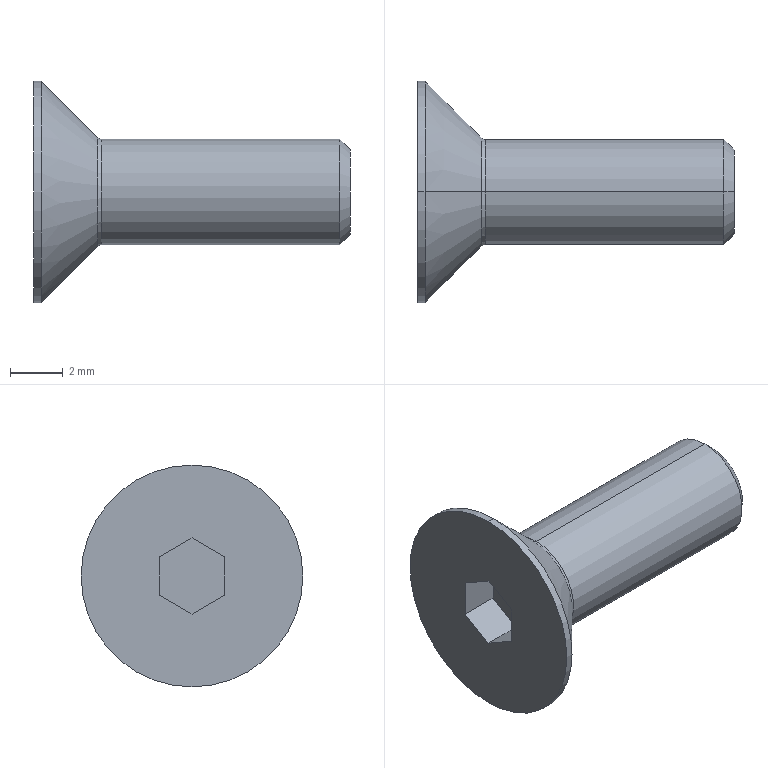Part | STEP file | 1 solid | 19 faces | box 12 x 8.4 x 8.4 mm | volume 195.31 mm3 | plane 9 | cylinder 4 | cone 4 | spline 2 | commonest cylinder face diameters 4 x2 8.4 x2
STEP:
#1=CARTESIAN_POINT('',(0.,0.,0.));
#2=DIRECTION('',(0.,0.,1.));
#3=DIRECTION('',(1.,0.,0.));
#4=AXIS2_PLACEMENT_3D('',#1,#2,#3);
#5=CARTESIAN_POINT('',(-0.98,-1.25,-0.7217));
#6=VERTEX_POINT('',#5);
#7=CARTESIAN_POINT('',(-0.98,-1.25,0.7217));
#8=VERTEX_POINT('',#7);
#9=CARTESIAN_POINT('',(-0.98,-1.25,-0.7217));
#10=DIRECTION('',(0.,0.,1.));
#11=VECTOR('',#10,1.);
#12=LINE('',#9,#11);
#13=CARTESIAN_POINT('',(-0.98,0.,0.));
#14=DIRECTION('',(-1.,0.,0.));
#15=DIRECTION('',(0.,0.,1.));
#16=AXIS2_PLACEMENT_3D('',#13,#14,#15);
#17=PLANE('',#16);
#18=CARTESIAN_POINT('',(-0.7217,-1.25));
#19=DIRECTION('',(1.,0.));
#20=VECTOR('',#19,1.);
#21=LINE('',#18,#20);
#22=(GEOMETRIC_REPRESENTATION_CONTEXT(2)PARAMETRIC_REPRESENTATION_CONTEXT()REPRESENTATION_CONTEXT('',''));
#23=DEFINITIONAL_REPRESENTATION('',(#21),#22);
#24=PCURVE('',#17,#23);
#25=CARTESIAN_POINT('',(-0.98,-1.25,-0.7217));
#26=DIRECTION('',(0.,-1.,0.));
#27=DIRECTION('',(-1.,0.,0.));
#28=AXIS2_PLACEMENT_3D('',#25,#26,#27);
#29=PLANE('',#28);
#30=CARTESIAN_POINT('',(0.,0.));
#31=DIRECTION('',(0.,-1.));
#32=VECTOR('',#31,1.);
#33=LINE('',#30,#32);
#34=(GEOMETRIC_REPRESENTATION_CONTEXT(2)PARAMETRIC_REPRESENTATION_CONTEXT()REPRESENTATION_CONTEXT('',''));
#35=DEFINITIONAL_REPRESENTATION('',(#33),#34);
#36=PCURVE('',#29,#35);
#37=SURFACE_CURVE('',#12,(#24,#36),.PCURVE_S1.);
#38=EDGE_CURVE('',#6,#8,#37,.T.);
#39=ORIENTED_EDGE('',*,*,#38,.T.);
#40=CARTESIAN_POINT('',(-0.98,0.,1.443));
#41=VERTEX_POINT('',#40);
#42=CARTESIAN_POINT('',(-0.98,-1.25,0.7217));
#43=DIRECTION('',(0.,0.866,0.5));
#44=VECTOR('',#43,1.);
#45=LINE('',#42,#44);
#46=CARTESIAN_POINT('',(0.7217,-1.25));
#47=DIRECTION('',(0.5,0.866));
#48=VECTOR('',#47,1.);
#49=LINE('',#46,#48);
#50=(GEOMETRIC_REPRESENTATION_CONTEXT(2)PARAMETRIC_REPRESENTATION_CONTEXT()REPRESENTATION_CONTEXT('',''));
#51=DEFINITIONAL_REPRESENTATION('',(#49),#50);
#52=PCURVE('',#17,#51);
#53=CARTESIAN_POINT('',(-0.98,-1.25,0.7217));
#54=DIRECTION('',(0.,-0.5,0.866));
#55=DIRECTION('',(-1.,0.,0.));
#56=AXIS2_PLACEMENT_3D('',#53,#54,#55);
#57=PLANE('',#56);
#58=CARTESIAN_POINT('',(0.,0.));
#59=DIRECTION('',(0.,-1.));
#60=VECTOR('',#59,1.);
#61=LINE('',#58,#60);
#62=(GEOMETRIC_REPRESENTATION_CONTEXT(2)PARAMETRIC_REPRESENTATION_CONTEXT()REPRESENTATION_CONTEXT('',''));
#63=DEFINITIONAL_REPRESENTATION('',(#61),#62);
#64=PCURVE('',#57,#63);
#65=SURFACE_CURVE('',#45,(#52,#64),.PCURVE_S1.);
#66=EDGE_CURVE('',#8,#41,#65,.T.);
#67=ORIENTED_EDGE('',*,*,#66,.T.);
#68=CARTESIAN_POINT('',(-0.98,1.25,0.7217));
#69=VERTEX_POINT('',#68);
#70=CARTESIAN_POINT('',(-0.98,0.,1.443));
#71=DIRECTION('',(0.,0.866,-0.5));
#72=VECTOR('',#71,1.);
#73=LINE('',#70,#72);
#74=CARTESIAN_POINT('',(1.443,0.));
#75=DIRECTION('',(-0.5,0.866));
#76=VECTOR('',#75,1.);
#77=LINE('',#74,#76);
#78=(GEOMETRIC_REPRESENTATION_CONTEXT(2)PARAMETRIC_REPRESENTATION_CONTEXT()REPRESENTATION_CONTEXT('',''));
#79=DEFINITIONAL_REPRESENTATION('',(#77),#78);
#80=PCURVE('',#17,#79);
#81=CARTESIAN_POINT('',(-0.98,0.,1.443));
#82=DIRECTION('',(0.,0.5,0.866));
#83=DIRECTION('',(1.,0.,0.));
#84=AXIS2_PLACEMENT_3D('',#81,#82,#83);
#85=PLANE('',#84);
#86=CARTESIAN_POINT('',(0.,0.));
#87=DIRECTION('',(0.,1.));
#88=VECTOR('',#87,1.);
#89=LINE('',#86,#88);
#90=(GEOMETRIC_REPRESENTATION_CONTEXT(2)PARAMETRIC_REPRESENTATION_CONTEXT()REPRESENTATION_CONTEXT('',''));
#91=DEFINITIONAL_REPRESENTATION('',(#89),#90);
#92=PCURVE('',#85,#91);
#93=SURFACE_CURVE('',#73,(#80,#92),.PCURVE_S1.);
#94=EDGE_CURVE('',#41,#69,#93,.T.);
#95=ORIENTED_EDGE('',*,*,#94,.T.);
#96=CARTESIAN_POINT('',(-0.98,1.25,-0.7217));
#97=VERTEX_POINT('',#96);
#98=CARTESIAN_POINT('',(-0.98,1.25,0.7217));
#99=DIRECTION('',(0.,0.,-1.));
#100=VECTOR('',#99,1.);
#101=LINE('',#98,#100);
#102=CARTESIAN_POINT('',(0.7217,1.25));
#103=DIRECTION('',(-1.,0.));
#104=VECTOR('',#103,1.);
#105=LINE('',#102,#104);
#106=(GEOMETRIC_REPRESENTATION_CONTEXT(2)PARAMETRIC_REPRESENTATION_CONTEXT()REPRESENTATION_CONTEXT('',''));
#107=DEFINITIONAL_REPRESENTATION('',(#105),#106);
#108=PCURVE('',#17,#107);
#109=CARTESIAN_POINT('',(-0.98,1.25,0.7217));
#110=DIRECTION('',(0.,1.,0.));
#111=DIRECTION('',(1.,0.,0.));
#112=AXIS2_PLACEMENT_3D('',#109,#110,#111);
#113=PLANE('',#112);
#114=CARTESIAN_POINT('',(0.,0.));
#115=DIRECTION('',(0.,1.));
#116=VECTOR('',#115,1.);
#117=LINE('',#114,#116);
#118=(GEOMETRIC_REPRESENTATION_CONTEXT(2)PARAMETRIC_REPRESENTATION_CONTEXT()REPRESENTATION_CONTEXT('',''));
#119=DEFINITIONAL_REPRESENTATION('',(#117),#118);
#120=PCURVE('',#113,#119);
#121=SURFACE_CURVE('',#101,(#108,#120),.PCURVE_S1.);
#122=EDGE_CURVE('',#69,#97,#121,.T.);
#123=ORIENTED_EDGE('',*,*,#122,.T.);
#124=CARTESIAN_POINT('',(-0.98,0.,-1.443));
#125=VERTEX_POINT('',#124);
#126=CARTESIAN_POINT('',(-0.98,1.25,-0.7217));
#127=DIRECTION('',(0.,-0.866,-0.5));
#128=VECTOR('',#127,1.);
#129=LINE('',#126,#128);
#130=CARTESIAN_POINT('',(-0.7217,1.25));
#131=DIRECTION('',(-0.5,-0.866));
#132=VECTOR('',#131,1.);
#133=LINE('',#130,#132);
#134=(GEOMETRIC_REPRESENTATION_CONTEXT(2)PARAMETRIC_REPRESENTATION_CONTEXT()REPRESENTATION_CONTEXT('',''));
#135=DEFINITIONAL_REPRESENTATION('',(#133),#134);
#136=PCURVE('',#17,#135);
#137=CARTESIAN_POINT('',(-0.98,1.25,-0.7217));
#138=DIRECTION('',(0.,0.5,-0.866));
#139=DIRECTION('',(-1.,0.,0.));
#140=AXIS2_PLACEMENT_3D('',#137,#138,#139);
#141=PLANE('',#140);
#142=CARTESIAN_POINT('',(0.,0.));
#143=DIRECTION('',(0.,-1.));
#144=VECTOR('',#143,1.);
#145=LINE('',#142,#144);
#146=(GEOMETRIC_REPRESENTATION_CONTEXT(2)PARAMETRIC_REPRESENTATION_CONTEXT()REPRESENTATION_CONTEXT('',''));
#147=DEFINITIONAL_REPRESENTATION('',(#145),#146);
#148=PCURVE('',#141,#147);
#149=SURFACE_CURVE('',#129,(#136,#148),.PCURVE_S1.);
#150=EDGE_CURVE('',#97,#125,#149,.T.);
#151=ORIENTED_EDGE('',*,*,#150,.T.);
#152=CARTESIAN_POINT('',(-0.98,0.,-1.443));
#153=DIRECTION('',(0.,-0.866,0.5));
#154=VECTOR('',#153,1.);
#155=LINE('',#152,#154);
#156=CARTESIAN_POINT('',(-1.443,0.));
#157=DIRECTION('',(0.5,-0.866));
#158=VECTOR('',#157,1.);
#159=LINE('',#156,#158);
#160=(GEOMETRIC_REPRESENTATION_CONTEXT(2)PARAMETRIC_REPRESENTATION_CONTEXT()REPRESENTATION_CONTEXT('',''));
#161=DEFINITIONAL_REPRESENTATION('',(#159),#160);
#162=PCURVE('',#17,#161);
#163=CARTESIAN_POINT('',(-0.98,0.,-1.443));
#164=DIRECTION('',(0.,-0.5,-0.866));
#165=DIRECTION('',(0.,-0.866,0.5));
#166=AXIS2_PLACEMENT_3D('',#163,#164,#165);
#167=PLANE('',#166);
#168=CARTESIAN_POINT('',(0.,0.));
#169=DIRECTION('',(1.,0.));
#170=VECTOR('',#169,1.);
#171=LINE('',#168,#170);
#172=(GEOMETRIC_REPRESENTATION_CONTEXT(2)PARAMETRIC_REPRESENTATION_CONTEXT()REPRESENTATION_CONTEXT('',''));
#173=DEFINITIONAL_REPRESENTATION('',(#171),#172);
#174=PCURVE('',#167,#173);
#175=SURFACE_CURVE('',#155,(#162,#174),.PCURVE_S1.);
#176=EDGE_CURVE('',#125,#6,#175,.T.);
#177=ORIENTED_EDGE('',*,*,#176,.T.);
#178=EDGE_LOOP('',(#39,#67,#95,#123,#151,#177));
#179=FACE_BOUND('',#178,.T.);
#180=ADVANCED_FACE('',(#179),#17,.T.);
#181=CARTESIAN_POINT('',(-2.48,0.,-1.443));
#182=VERTEX_POINT('',#181);
#183=CARTESIAN_POINT('',(-0.98,0.,-1.443));
#184=DIRECTION('',(1.,0.,0.));
#185=VECTOR('',#184,1.);
#186=LINE('',#183,#185);
#187=CARTESIAN_POINT('',(0.,-1.443));
#188=DIRECTION('',(-1.,0.));
#189=VECTOR('',#188,1.);
#190=LINE('',#187,#189);
#191=(GEOMETRIC_REPRESENTATION_CONTEXT(2)PARAMETRIC_REPRESENTATION_CONTEXT()REPRESENTATION_CONTEXT('',''));
#192=DEFINITIONAL_REPRESENTATION('',(#190),#191);
#193=PCURVE('',#141,#192);
#194=CARTESIAN_POINT('',(0.,0.));
#195=DIRECTION('',(0.,-1.));
#196=VECTOR('',#195,1.);
#197=LINE('',#194,#196);
#198=(GEOMETRIC_REPRESENTATION_CONTEXT(2)PARAMETRIC_REPRESENTATION_CONTEXT()REPRESENTATION_CONTEXT('',''));
#199=DEFINITIONAL_REPRESENTATION('',(#197),#198);
#200=PCURVE('',#167,#199);
#201=SURFACE_CURVE('',#186,(#193,#200),.PCURVE_S1.);
#202=EDGE_CURVE('',#182,#125,#201,.T.);
#203=ORIENTED_EDGE('',*,*,#202,.T.);
#204=ORIENTED_EDGE('',*,*,#150,.F.);
#205=CARTESIAN_POINT('',(-2.48,1.25,-0.7217));
#206=VERTEX_POINT('',#205);
#207=CARTESIAN_POINT('',(-0.98,1.25,-0.7217));
#208=DIRECTION('',(-1.,0.,0.));
#209=VECTOR('',#208,1.);
#210=LINE('',#207,#209);
#211=CARTESIAN_POINT('',(0.,0.));
#212=DIRECTION('',(1.,0.));
#213=VECTOR('',#212,1.);
#214=LINE('',#211,#213);
#215=(GEOMETRIC_REPRESENTATION_CONTEXT(2)PARAMETRIC_REPRESENTATION_CONTEXT()REPRESENTATION_CONTEXT('',''));
#216=DEFINITIONAL_REPRESENTATION('',(#214),#215);
#217=PCURVE('',#141,#216);
#218=CARTESIAN_POINT('',(0.,1.443));
#219=DIRECTION('',(-1.,0.));
#220=VECTOR('',#219,1.);
#221=LINE('',#218,#220);
#222=(GEOMETRIC_REPRESENTATION_CONTEXT(2)PARAMETRIC_REPRESENTATION_CONTEXT()REPRESENTATION_CONTEXT('',''));
#223=DEFINITIONAL_REPRESENTATION('',(#221),#222);
#224=PCURVE('',#113,#223);
#225=SURFACE_CURVE('',#210,(#217,#224),.PCURVE_S1.);
#226=EDGE_CURVE('',#97,#206,#225,.T.);
#227=ORIENTED_EDGE('',*,*,#226,.T.);
#228=CARTESIAN_POINT('',(-2.48,1.25,-0.7217));
#229=DIRECTION('',(0.,-0.866,-0.5));
#230=VECTOR('',#229,1.);
#231=LINE('',#228,#230);
#232=CARTESIAN_POINT('',(1.5,0.));
#233=DIRECTION('',(0.,-1.));
#234=VECTOR('',#233,1.);
#235=LINE('',#232,#234);
#236=(GEOMETRIC_REPRESENTATION_CONTEXT(2)PARAMETRIC_REPRESENTATION_CONTEXT()REPRESENTATION_CONTEXT('',''));
#237=DEFINITIONAL_REPRESENTATION('',(#235),#236);
#238=PCURVE('',#141,#237);
#239=CARTESIAN_POINT('',(-2.48,4.2,0.));
#240=DIRECTION('',(1.,0.,0.));
#241=DIRECTION('',(0.,1.,0.));
#242=AXIS2_PLACEMENT_3D('',#239,#240,#241);
#243=PLANE('',#242);
#244=CARTESIAN_POINT('',(-2.95,-0.7217));
#245=DIRECTION('',(-0.866,-0.5));
#246=VECTOR('',#245,1.);
#247=LINE('',#244,#246);
#248=(GEOMETRIC_REPRESENTATION_CONTEXT(2)PARAMETRIC_REPRESENTATION_CONTEXT()REPRESENTATION_CONTEXT('',''));
#249=DEFINITIONAL_REPRESENTATION('',(#247),#248);
#250=PCURVE('',#243,#249);
#251=SURFACE_CURVE('',#231,(#238,#250),.PCURVE_S1.);
#252=EDGE_CURVE('',#206,#182,#251,.T.);
#253=ORIENTED_EDGE('',*,*,#252,.T.);
#254=EDGE_LOOP('',(#203,#204,#227,#253));
#255=FACE_BOUND('',#254,.T.);
#256=ADVANCED_FACE('',(#255),#141,.F.);
#257=CARTESIAN_POINT('',(-2.48,-1.25,-0.7217));
#258=VERTEX_POINT('',#257);
#259=CARTESIAN_POINT('',(-0.98,-1.25,-0.7217));
#260=DIRECTION('',(1.,0.,0.));
#261=VECTOR('',#260,1.);
#262=LINE('',#259,#261);
#263=CARTESIAN_POINT('',(1.443,0.));
#264=DIRECTION('',(0.,-1.));
#265=VECTOR('',#264,1.);
#266=LINE('',#263,#265);
#267=(GEOMETRIC_REPRESENTATION_CONTEXT(2)PARAMETRIC_REPRESENTATION_CONTEXT()REPRESENTATION_CONTEXT('',''));
#268=DEFINITIONAL_REPRESENTATION('',(#266),#267);
#269=PCURVE('',#167,#268);
#270=CARTESIAN_POINT('',(0.,0.));
#271=DIRECTION('',(-1.,0.));
#272=VECTOR('',#271,1.);
#273=LINE('',#270,#272);
#274=(GEOMETRIC_REPRESENTATION_CONTEXT(2)PARAMETRIC_REPRESENTATION_CONTEXT()REPRESENTATION_CONTEXT('',''));
#275=DEFINITIONAL_REPRESENTATION('',(#273),#274);
#276=PCURVE('',#29,#275);
#277=SURFACE_CURVE('',#262,(#269,#276),.PCURVE_S1.);
#278=EDGE_CURVE('',#258,#6,#277,.T.);
#279=ORIENTED_EDGE('',*,*,#278,.T.);
#280=ORIENTED_EDGE('',*,*,#176,.F.);
#281=ORIENTED_EDGE('',*,*,#202,.F.);
#282=CARTESIAN_POINT('',(-2.48,0.,-1.443));
#283=DIRECTION('',(0.,-0.866,0.5));
#284=VECTOR('',#283,1.);
#285=LINE('',#282,#284);
#286=CARTESIAN_POINT('',(0.,1.5));
#287=DIRECTION('',(1.,0.));
#288=VECTOR('',#287,1.);
#289=LINE('',#286,#288);
#290=(GEOMETRIC_REPRESENTATION_CONTEXT(2)PARAMETRIC_REPRESENTATION_CONTEXT()REPRESENTATION_CONTEXT('',''));
#291=DEFINITIONAL_REPRESENTATION('',(#289),#290);
#292=PCURVE('',#167,#291);
#293=CARTESIAN_POINT('',(-4.2,-1.443));
#294=DIRECTION('',(-0.866,0.5));
#295=VECTOR('',#294,1.);
#296=LINE('',#293,#295);
#297=(GEOMETRIC_REPRESENTATION_CONTEXT(2)PARAMETRIC_REPRESENTATION_CONTEXT()REPRESENTATION_CONTEXT('',''));
#298=DEFINITIONAL_REPRESENTATION('',(#296),#297);
#299=PCURVE('',#243,#298);
#300=SURFACE_CURVE('',#285,(#292,#299),.PCURVE_S1.);
#301=EDGE_CURVE('',#182,#258,#300,.T.);
#302=ORIENTED_EDGE('',*,*,#301,.T.);
#303=EDGE_LOOP('',(#279,#280,#281,#302));
#304=FACE_BOUND('',#303,.T.);
#305=ADVANCED_FACE('',(#304),#167,.F.);
#306=CARTESIAN_POINT('',(-2.48,-1.25,0.7217));
#307=VERTEX_POINT('',#306);
#308=CARTESIAN_POINT('',(-0.98,-1.25,0.7217));
#309=DIRECTION('',(1.,0.,0.));
#310=VECTOR('',#309,1.);
#311=LINE('',#308,#310);
#312=CARTESIAN_POINT('',(0.,-1.443));
#313=DIRECTION('',(-1.,0.));
#314=VECTOR('',#313,1.);
#315=LINE('',#312,#314);
#316=(GEOMETRIC_REPRESENTATION_CONTEXT(2)PARAMETRIC_REPRESENTATION_CONTEXT()REPRESENTATION_CONTEXT('',''));
#317=DEFINITIONAL_REPRESENTATION('',(#315),#316);
#318=PCURVE('',#29,#317);
#319=CARTESIAN_POINT('',(0.,0.));
#320=DIRECTION('',(-1.,0.));
#321=VECTOR('',#320,1.);
#322=LINE('',#319,#321);
#323=(GEOMETRIC_REPRESENTATION_CONTEXT(2)PARAMETRIC_REPRESENTATION_CONTEXT()REPRESENTATION_CONTEXT('',''));
#324=DEFINITIONAL_REPRESENTATION('',(#322),#323);
#325=PCURVE('',#57,#324);
#326=SURFACE_CURVE('',#311,(#318,#325),.PCURVE_S1.);
#327=EDGE_CURVE('',#307,#8,#326,.T.);
#328=ORIENTED_EDGE('',*,*,#327,.T.);
#329=ORIENTED_EDGE('',*,*,#38,.F.);
#330=ORIENTED_EDGE('',*,*,#278,.F.);
#331=CARTESIAN_POINT('',(-2.48,-1.25,0.));
#332=DIRECTION('',(0.,0.,1.));
#333=VECTOR('',#332,1.);
#334=LINE('',#331,#333);
#335=CARTESIAN_POINT('',(1.5,-0.7217));
#336=DIRECTION('',(0.,-1.));
#337=VECTOR('',#336,1.);
#338=LINE('',#335,#337);
#339=(GEOMETRIC_REPRESENTATION_CONTEXT(2)PARAMETRIC_REPRESENTATION_CONTEXT()REPRESENTATION_CONTEXT('',''));
#340=DEFINITIONAL_REPRESENTATION('',(#338),#339);
#341=PCURVE('',#29,#340);
#342=CARTESIAN_POINT('',(-5.45,0.));
#343=DIRECTION('',(0.,1.));
#344=VECTOR('',#343,1.);
#345=LINE('',#342,#344);
#346=(GEOMETRIC_REPRESENTATION_CONTEXT(2)PARAMETRIC_REPRESENTATION_CONTEXT()REPRESENTATION_CONTEXT('',''));
#347=DEFINITIONAL_REPRESENTATION('',(#345),#346);
#348=PCURVE('',#243,#347);
#349=SURFACE_CURVE('',#334,(#341,#348),.PCURVE_S1.);
#350=EDGE_CURVE('',#258,#307,#349,.T.);
#351=ORIENTED_EDGE('',*,*,#350,.T.);
#352=EDGE_LOOP('',(#328,#329,#330,#351));
#353=FACE_BOUND('',#352,.T.);
#354=ADVANCED_FACE('',(#353),#29,.F.);
#355=CARTESIAN_POINT('',(-2.48,0.,1.443));
#356=VERTEX_POINT('',#355);
#357=CARTESIAN_POINT('',(-0.98,0.,1.443));
#358=DIRECTION('',(1.,0.,0.));
#359=VECTOR('',#358,1.);
#360=LINE('',#357,#359);
#361=CARTESIAN_POINT('',(0.,-1.443));
#362=DIRECTION('',(-1.,0.));
#363=VECTOR('',#362,1.);
#364=LINE('',#361,#363);
#365=(GEOMETRIC_REPRESENTATION_CONTEXT(2)PARAMETRIC_REPRESENTATION_CONTEXT()REPRESENTATION_CONTEXT('',''));
#366=DEFINITIONAL_REPRESENTATION('',(#364),#365);
#367=PCURVE('',#57,#366);
#368=CARTESIAN_POINT('',(0.,0.));
#369=DIRECTION('',(1.,0.));
#370=VECTOR('',#369,1.);
#371=LINE('',#368,#370);
#372=(GEOMETRIC_REPRESENTATION_CONTEXT(2)PARAMETRIC_REPRESENTATION_CONTEXT()REPRESENTATION_CONTEXT('',''));
#373=DEFINITIONAL_REPRESENTATION('',(#371),#372);
#374=PCURVE('',#85,#373);
#375=SURFACE_CURVE('',#360,(#367,#374),.PCURVE_S1.);
#376=EDGE_CURVE('',#356,#41,#375,.T.);
#377=ORIENTED_EDGE('',*,*,#376,.T.);
#378=ORIENTED_EDGE('',*,*,#66,.F.);
#379=ORIENTED_EDGE('',*,*,#327,.F.);
#380=CARTESIAN_POINT('',(-2.48,-1.25,0.7217));
#381=DIRECTION('',(0.,0.866,0.5));
#382=VECTOR('',#381,1.);
#383=LINE('',#380,#382);
#384=CARTESIAN_POINT('',(1.5,0.));
#385=DIRECTION('',(0.,-1.));
#386=VECTOR('',#385,1.);
#387=LINE('',#384,#386);
#388=(GEOMETRIC_REPRESENTATION_CONTEXT(2)PARAMETRIC_REPRESENTATION_CONTEXT()REPRESENTATION_CONTEXT('',''));
#389=DEFINITIONAL_REPRESENTATION('',(#387),#388);
#390=PCURVE('',#57,#389);
#391=CARTESIAN_POINT('',(-5.45,0.7217));
#392=DIRECTION('',(0.866,0.5));
#393=VECTOR('',#392,1.);
#394=LINE('',#391,#393);
#395=(GEOMETRIC_REPRESENTATION_CONTEXT(2)PARAMETRIC_REPRESENTATION_CONTEXT()REPRESENTATION_CONTEXT('',''));
#396=DEFINITIONAL_REPRESENTATION('',(#394),#395);
#397=PCURVE('',#243,#396);
#398=SURFACE_CURVE('',#383,(#390,#397),.PCURVE_S1.);
#399=EDGE_CURVE('',#307,#356,#398,.T.);
#400=ORIENTED_EDGE('',*,*,#399,.T.);
#401=EDGE_LOOP('',(#377,#378,#379,#400));
#402=FACE_BOUND('',#401,.T.);
#403=ADVANCED_FACE('',(#402),#57,.F.);
#404=CARTESIAN_POINT('',(-2.48,1.25,0.7217));
#405=VERTEX_POINT('',#404);
#406=CARTESIAN_POINT('',(-0.98,1.25,0.7217));
#407=DIRECTION('',(1.,0.,0.));
#408=VECTOR('',#407,1.);
#409=LINE('',#406,#408);
#410=CARTESIAN_POINT('',(0.,1.443));
#411=DIRECTION('',(1.,0.));
#412=VECTOR('',#411,1.);
#413=LINE('',#410,#412);
#414=(GEOMETRIC_REPRESENTATION_CONTEXT(2)PARAMETRIC_REPRESENTATION_CONTEXT()REPRESENTATION_CONTEXT('',''));
#415=DEFINITIONAL_REPRESENTATION('',(#413),#414);
#416=PCURVE('',#85,#415);
#417=CARTESIAN_POINT('',(0.,0.));
#418=DIRECTION('',(1.,0.));
#419=VECTOR('',#418,1.);
#420=LINE('',#417,#419);
#421=(GEOMETRIC_REPRESENTATION_CONTEXT(2)PARAMETRIC_REPRESENTATION_CONTEXT()REPRESENTATION_CONTEXT('',''));
#422=DEFINITIONAL_REPRESENTATION('',(#420),#421);
#423=PCURVE('',#113,#422);
#424=SURFACE_CURVE('',#409,(#416,#423),.PCURVE_S1.);
#425=EDGE_CURVE('',#405,#69,#424,.T.);
#426=ORIENTED_EDGE('',*,*,#425,.T.);
#427=ORIENTED_EDGE('',*,*,#94,.F.);
#428=ORIENTED_EDGE('',*,*,#376,.F.);
#429=CARTESIAN_POINT('',(-2.48,0.,1.443));
#430=DIRECTION('',(0.,0.866,-0.5));
#431=VECTOR('',#430,1.);
#432=LINE('',#429,#431);
#433=CARTESIAN_POINT('',(-1.5,0.));
#434=DIRECTION('',(0.,1.));
#435=VECTOR('',#434,1.);
#436=LINE('',#433,#435);
#437=(GEOMETRIC_REPRESENTATION_CONTEXT(2)PARAMETRIC_REPRESENTATION_CONTEXT()REPRESENTATION_CONTEXT('',''));
#438=DEFINITIONAL_REPRESENTATION('',(#436),#437);
#439=PCURVE('',#85,#438);
#440=CARTESIAN_POINT('',(-4.2,1.443));
#441=DIRECTION('',(0.866,-0.5));
#442=VECTOR('',#441,1.);
#443=LINE('',#440,#442);
#444=(GEOMETRIC_REPRESENTATION_CONTEXT(2)PARAMETRIC_REPRESENTATION_CONTEXT()REPRESENTATION_CONTEXT('',''));
#445=DEFINITIONAL_REPRESENTATION('',(#443),#444);
#446=PCURVE('',#243,#445);
#447=SURFACE_CURVE('',#432,(#439,#446),.PCURVE_S1.);
#448=EDGE_CURVE('',#356,#405,#447,.T.);
#449=ORIENTED_EDGE('',*,*,#448,.T.);
#450=EDGE_LOOP('',(#426,#427,#428,#449));
#451=FACE_BOUND('',#450,.T.);
#452=ADVANCED_FACE('',(#451),#85,.F.);
#453=ORIENTED_EDGE('',*,*,#226,.F.);
#454=ORIENTED_EDGE('',*,*,#122,.F.);
#455=ORIENTED_EDGE('',*,*,#425,.F.);
#456=CARTESIAN_POINT('',(-2.48,1.25,0.));
#457=DIRECTION('',(0.,0.,-1.));
#458=VECTOR('',#457,1.);
#459=LINE('',#456,#458);
#460=CARTESIAN_POINT('',(-1.5,0.7217));
#461=DIRECTION('',(0.,1.));
#462=VECTOR('',#461,1.);
#463=LINE('',#460,#462);
#464=(GEOMETRIC_REPRESENTATION_CONTEXT(2)PARAMETRIC_REPRESENTATION_CONTEXT()REPRESENTATION_CONTEXT('',''));
#465=DEFINITIONAL_REPRESENTATION('',(#463),#464);
#466=PCURVE('',#113,#465);
#467=CARTESIAN_POINT('',(-2.95,0.));
#468=DIRECTION('',(0.,-1.));
#469=VECTOR('',#468,1.);
#470=LINE('',#467,#469);
#471=(GEOMETRIC_REPRESENTATION_CONTEXT(2)PARAMETRIC_REPRESENTATION_CONTEXT()REPRESENTATION_CONTEXT('',''));
#472=DEFINITIONAL_REPRESENTATION('',(#470),#471);
#473=PCURVE('',#243,#472);
#474=SURFACE_CURVE('',#459,(#466,#473),.PCURVE_S1.);
#475=EDGE_CURVE('',#405,#206,#474,.T.);
#476=ORIENTED_EDGE('',*,*,#475,.T.);
#477=EDGE_LOOP('',(#453,#454,#455,#476));
#478=FACE_BOUND('',#477,.T.);
#479=ADVANCED_FACE('',(#478),#113,.F.);
#480=ORIENTED_EDGE('',*,*,#448,.F.);
#481=ORIENTED_EDGE('',*,*,#399,.F.);
#482=ORIENTED_EDGE('',*,*,#350,.F.);
#483=ORIENTED_EDGE('',*,*,#301,.F.);
#484=ORIENTED_EDGE('',*,*,#252,.F.);
#485=ORIENTED_EDGE('',*,*,#475,.F.);
#486=EDGE_LOOP('',(#480,#481,#482,#483,#484,#485));
#487=FACE_BOUND('',#486,.T.);
#488=CARTESIAN_POINT('',(-2.48,0.,4.2));
#489=VERTEX_POINT('',#488);
#490=CARTESIAN_POINT('',(-2.48,0.,-4.2));
#491=VERTEX_POINT('',#490);
#492=CARTESIAN_POINT('',(-2.48,0.,0.));
#493=DIRECTION('',(1.,0.,0.));
#494=DIRECTION('',(0.,0.,1.));
#495=AXIS2_PLACEMENT_3D('',#492,#493,#494);
#496=CIRCLE('',#495,4.2);
#497=CARTESIAN_POINT('',(-4.2,0.));
#498=DIRECTION('',(0.,1.));
#499=AXIS2_PLACEMENT_2D('',#497,#498);
#500=CIRCLE('',#499,4.2);
#501=(GEOMETRIC_REPRESENTATION_CONTEXT(2)PARAMETRIC_REPRESENTATION_CONTEXT()REPRESENTATION_CONTEXT('',''));
#502=DEFINITIONAL_REPRESENTATION('',(#500),#501);
#503=PCURVE('',#243,#502);
#504=CARTESIAN_POINT('',(-21.552,0.,0.));
#505=DIRECTION('',(-1.,0.,0.));
#506=DIRECTION('',(0.,0.,1.));
#507=AXIS2_PLACEMENT_3D('',#504,#505,#506);
#508=CYLINDRICAL_SURFACE('',#507,4.2);
#509=CARTESIAN_POINT('',(6.283,-19.072));
#510=DIRECTION('',(-1.,0.));
#511=VECTOR('',#510,1.);
#512=LINE('',#509,#511);
#513=(GEOMETRIC_REPRESENTATION_CONTEXT(2)PARAMETRIC_REPRESENTATION_CONTEXT()REPRESENTATION_CONTEXT('',''));
#514=DEFINITIONAL_REPRESENTATION('',(#512),#513);
#515=PCURVE('',#508,#514);
#516=SURFACE_CURVE('',#496,(#503,#515),.PCURVE_S1.);
#517=EDGE_CURVE('',#489,#491,#516,.T.);
#518=ORIENTED_EDGE('',*,*,#517,.F.);
#519=CARTESIAN_POINT('',(-2.48,0.,0.));
#520=DIRECTION('',(1.,0.,0.));
#521=DIRECTION('',(0.,0.,1.));
#522=AXIS2_PLACEMENT_3D('',#519,#520,#521);
#523=CIRCLE('',#522,4.2);
#524=CARTESIAN_POINT('',(-4.2,0.));
#525=DIRECTION('',(0.,1.));
#526=AXIS2_PLACEMENT_2D('',#524,#525);
#527=CIRCLE('',#526,4.2);
#528=(GEOMETRIC_REPRESENTATION_CONTEXT(2)PARAMETRIC_REPRESENTATION_CONTEXT()REPRESENTATION_CONTEXT('',''));
#529=DEFINITIONAL_REPRESENTATION('',(#527),#528);
#530=PCURVE('',#243,#529);
#531=CARTESIAN_POINT('',(-21.552,0.,0.));
#532=DIRECTION('',(-1.,0.,0.));
#533=DIRECTION('',(0.,0.,1.));
#534=AXIS2_PLACEMENT_3D('',#531,#532,#533);
#535=CYLINDRICAL_SURFACE('',#534,4.2);
#536=CARTESIAN_POINT('',(6.283,-19.072));
#537=DIRECTION('',(-1.,0.));
#538=VECTOR('',#537,1.);
#539=LINE('',#536,#538);
#540=(GEOMETRIC_REPRESENTATION_CONTEXT(2)PARAMETRIC_REPRESENTATION_CONTEXT()REPRESENTATION_CONTEXT('',''));
#541=DEFINITIONAL_REPRESENTATION('',(#539),#540);
#542=PCURVE('',#535,#541);
#543=SURFACE_CURVE('',#523,(#530,#542),.PCURVE_S1.);
#544=EDGE_CURVE('',#491,#489,#543,.T.);
#545=ORIENTED_EDGE('',*,*,#544,.F.);
#546=EDGE_LOOP('',(#518,#545));
#547=FACE_BOUND('',#546,.T.);
#548=ADVANCED_FACE('',(#487,#547),#243,.F.);
#549=CARTESIAN_POINT('',(-2.2,0.,-4.2));
#550=VERTEX_POINT('',#549);
#551=CARTESIAN_POINT('',(-21.552,0.,-4.2));
#552=DIRECTION('',(-1.,0.,0.));
#553=VECTOR('',#552,1.);
#554=LINE('',#551,#553);
#555=CARTESIAN_POINT('',(3.142,0.));
#556=DIRECTION('',(0.,1.));
#557=VECTOR('',#556,1.);
#558=LINE('',#555,#557);
#559=(GEOMETRIC_REPRESENTATION_CONTEXT(2)PARAMETRIC_REPRESENTATION_CONTEXT()REPRESENTATION_CONTEXT('',''));
#560=DEFINITIONAL_REPRESENTATION('',(#558),#559);
#561=PCURVE('',#508,#560);
#562=CARTESIAN_POINT('',(3.142,0.));
#563=DIRECTION('',(0.,1.));
#564=VECTOR('',#563,1.);
#565=LINE('',#562,#564);
#566=(GEOMETRIC_REPRESENTATION_CONTEXT(2)PARAMETRIC_REPRESENTATION_CONTEXT()REPRESENTATION_CONTEXT('',''));
#567=DEFINITIONAL_REPRESENTATION('',(#565),#566);
#568=PCURVE('',#535,#567);
#569=SURFACE_CURVE('',#554,(#561,#568),.PCURVE_S1.);
#570=EDGE_CURVE('',#550,#491,#569,.T.);
#571=ORIENTED_EDGE('',*,*,#570,.F.);
#572=CARTESIAN_POINT('',(-2.2,0.,4.2));
#573=VERTEX_POINT('',#572);
#574=CARTESIAN_POINT('',(-2.2,0.,0.));
#575=DIRECTION('',(1.,0.,0.));
#576=DIRECTION('',(0.,0.,1.));
#577=AXIS2_PLACEMENT_3D('',#574,#575,#576);
#578=CIRCLE('',#577,4.2);
#579=CARTESIAN_POINT('',(6.283,-19.352));
#580=DIRECTION('',(-1.,0.));
#581=VECTOR('',#580,1.);
#582=LINE('',#579,#581);
#583=(GEOMETRIC_REPRESENTATION_CONTEXT(2)PARAMETRIC_REPRESENTATION_CONTEXT()REPRESENTATION_CONTEXT('',''));
#584=DEFINITIONAL_REPRESENTATION('',(#582),#583);
#585=PCURVE('',#508,#584);
#586=CARTESIAN_POINT('',(-2.2,0.,0.));
#587=DIRECTION('',(-1.,0.,0.));
#588=DIRECTION('',(0.,0.,1.));
#589=AXIS2_PLACEMENT_3D('',#586,#587,#588);
#590=CONICAL_SURFACE('',#589,4.2,0.7854);
#591=CARTESIAN_POINT('',(6.283,0.));
#592=DIRECTION('',(-1.,0.));
#593=VECTOR('',#592,1.);
#594=LINE('',#591,#593);
#595=(GEOMETRIC_REPRESENTATION_CONTEXT(2)PARAMETRIC_REPRESENTATION_CONTEXT()REPRESENTATION_CONTEXT('',''));
#596=DEFINITIONAL_REPRESENTATION('',(#594),#595);
#597=PCURVE('',#590,#596);
#598=SURFACE_CURVE('',#578,(#585,#597),.PCURVE_S1.);
#599=EDGE_CURVE('',#573,#550,#598,.T.);
#600=ORIENTED_EDGE('',*,*,#599,.F.);
#601=CARTESIAN_POINT('',(-21.552,0.,4.2));
#602=DIRECTION('',(-1.,0.,0.));
#603=VECTOR('',#602,1.);
#604=LINE('',#601,#603);
#605=CARTESIAN_POINT('',(6.283,0.));
#606=DIRECTION('',(0.,1.));
#607=VECTOR('',#606,1.);
#608=LINE('',#605,#607);
#609=(GEOMETRIC_REPRESENTATION_CONTEXT(2)PARAMETRIC_REPRESENTATION_CONTEXT()REPRESENTATION_CONTEXT('',''));
#610=DEFINITIONAL_REPRESENTATION('',(#608),#609);
#611=PCURVE('',#508,#610);
#612=CARTESIAN_POINT('',(0.,0.));
#613=DIRECTION('',(0.,1.));
#614=VECTOR('',#613,1.);
#615=LINE('',#612,#614);
#616=(GEOMETRIC_REPRESENTATION_CONTEXT(2)PARAMETRIC_REPRESENTATION_CONTEXT()REPRESENTATION_CONTEXT('',''));
#617=DEFINITIONAL_REPRESENTATION('',(#615),#616);
#618=PCURVE('',#535,#617);
#619=SURFACE_CURVE('',#604,(#611,#618),.PCURVE_S1.);
#620=EDGE_CURVE('',#573,#489,#619,.T.);
#621=ORIENTED_EDGE('',*,*,#620,.T.);
#622=ORIENTED_EDGE('',*,*,#517,.T.);
#623=EDGE_LOOP('',(#571,#600,#621,#622));
#624=FACE_BOUND('',#623,.T.);
#625=ADVANCED_FACE('',(#624),#508,.T.);
#626=CARTESIAN_POINT('',(9.52,0.,1.6));
#627=VERTEX_POINT('',#626);
#628=CARTESIAN_POINT('',(9.52,0.,-1.6));
#629=VERTEX_POINT('',#628);
#630=CARTESIAN_POINT('',(9.52,0.,0.));
#631=DIRECTION('',(-1.,0.,0.));
#632=DIRECTION('',(0.,0.,1.));
#633=AXIS2_PLACEMENT_3D('',#630,#631,#632);
#634=CIRCLE('',#633,1.6);
#635=CARTESIAN_POINT('',(9.52,2.,0.));
#636=DIRECTION('',(-1.,0.,0.));
#637=DIRECTION('',(0.,0.,1.));
#638=AXIS2_PLACEMENT_3D('',#635,#636,#637);
#639=PLANE('',#638);
#640=CARTESIAN_POINT('',(0.,-2.));
#641=DIRECTION('',(1.,0.));
#642=AXIS2_PLACEMENT_2D('',#640,#641);
#643=CIRCLE('',#642,1.6);
#644=(GEOMETRIC_REPRESENTATION_CONTEXT(2)PARAMETRIC_REPRESENTATION_CONTEXT()REPRESENTATION_CONTEXT('',''));
#645=DEFINITIONAL_REPRESENTATION('',(#643),#644);
#646=PCURVE('',#639,#645);
#647=CARTESIAN_POINT('',(9.12,0.,0.));
#648=DIRECTION('',(-1.,0.,0.));
#649=DIRECTION('',(0.,0.,1.));
#650=AXIS2_PLACEMENT_3D('',#647,#648,#649);
#651=CONICAL_SURFACE('',#650,2.,0.7854);
#652=CARTESIAN_POINT('',(0.,-0.4));
#653=DIRECTION('',(1.,0.));
#654=VECTOR('',#653,1.);
#655=LINE('',#652,#654);
#656=(GEOMETRIC_REPRESENTATION_CONTEXT(2)PARAMETRIC_REPRESENTATION_CONTEXT()REPRESENTATION_CONTEXT('',''));
#657=DEFINITIONAL_REPRESENTATION('',(#655),#656);
#658=PCURVE('',#651,#657);
#659=SURFACE_CURVE('',#634,(#646,#658),.PCURVE_S1.);
#660=EDGE_CURVE('',#627,#629,#659,.T.);
#661=ORIENTED_EDGE('',*,*,#660,.F.);
#662=CARTESIAN_POINT('',(9.52,0.,0.));
#663=DIRECTION('',(-1.,0.,0.));
#664=DIRECTION('',(0.,0.,1.));
#665=AXIS2_PLACEMENT_3D('',#662,#663,#664);
#666=CIRCLE('',#665,1.6);
#667=CARTESIAN_POINT('',(0.,-2.));
#668=DIRECTION('',(1.,0.));
#669=AXIS2_PLACEMENT_2D('',#667,#668);
#670=CIRCLE('',#669,1.6);
#671=(GEOMETRIC_REPRESENTATION_CONTEXT(2)PARAMETRIC_REPRESENTATION_CONTEXT()REPRESENTATION_CONTEXT('',''));
#672=DEFINITIONAL_REPRESENTATION('',(#670),#671);
#673=PCURVE('',#639,#672);
#674=CARTESIAN_POINT('',(9.12,0.,0.));
#675=DIRECTION('',(-1.,0.,0.));
#676=DIRECTION('',(0.,0.,1.));
#677=AXIS2_PLACEMENT_3D('',#674,#675,#676);
#678=CONICAL_SURFACE('',#677,2.,0.7854);
#679=CARTESIAN_POINT('',(0.,-0.4));
#680=DIRECTION('',(1.,0.));
#681=VECTOR('',#680,1.);
#682=LINE('',#679,#681);
#683=(GEOMETRIC_REPRESENTATION_CONTEXT(2)PARAMETRIC_REPRESENTATION_CONTEXT()REPRESENTATION_CONTEXT('',''));
#684=DEFINITIONAL_REPRESENTATION('',(#682),#683);
#685=PCURVE('',#678,#684);
#686=SURFACE_CURVE('',#666,(#673,#685),.PCURVE_S1.);
#687=EDGE_CURVE('',#629,#627,#686,.T.);
#688=ORIENTED_EDGE('',*,*,#687,.F.);
#689=EDGE_LOOP('',(#661,#688));
#690=FACE_BOUND('',#689,.T.);
#691=ADVANCED_FACE('',(#690),#639,.F.);
#692=CARTESIAN_POINT('',(-0.05858,0.,-2.059));
#693=VERTEX_POINT('',#692);
#694=CARTESIAN_POINT('',(-2.2,0.,-4.2));
#695=DIRECTION('',(-0.7071,0.,-0.7071));
#696=VECTOR('',#695,1.);
#697=LINE('',#694,#696);
#698=CARTESIAN_POINT('',(3.142,0.));
#699=DIRECTION('',(0.,1.));
#700=VECTOR('',#699,1.);
#701=LINE('',#698,#700);
#702=(GEOMETRIC_REPRESENTATION_CONTEXT(2)PARAMETRIC_REPRESENTATION_CONTEXT()REPRESENTATION_CONTEXT('',''));
#703=DEFINITIONAL_REPRESENTATION('',(#701),#702);
#704=PCURVE('',#590,#703);
#705=CARTESIAN_POINT('',(-2.2,0.,0.));
#706=DIRECTION('',(-1.,0.,0.));
#707=DIRECTION('',(0.,0.,1.));
#708=AXIS2_PLACEMENT_3D('',#705,#706,#707);
#709=CONICAL_SURFACE('',#708,4.2,0.7854);
#710=CARTESIAN_POINT('',(3.142,0.));
#711=DIRECTION('',(0.,1.));
#712=VECTOR('',#711,1.);
#713=LINE('',#710,#712);
#714=(GEOMETRIC_REPRESENTATION_CONTEXT(2)PARAMETRIC_REPRESENTATION_CONTEXT()REPRESENTATION_CONTEXT('',''));
#715=DEFINITIONAL_REPRESENTATION('',(#713),#714);
#716=PCURVE('',#709,#715);
#717=SURFACE_CURVE('',#697,(#704,#716),.PCURVE_S1.);
#718=EDGE_CURVE('',#693,#550,#717,.T.);
#719=ORIENTED_EDGE('',*,*,#718,.F.);
#720=CARTESIAN_POINT('',(-0.05858,0.,2.059));
#721=VERTEX_POINT('',#720);
#722=CARTESIAN_POINT('',(-0.05858,0.,0.));
#723=DIRECTION('',(-1.,0.,0.));
#724=DIRECTION('',(0.,0.,1.));
#725=AXIS2_PLACEMENT_3D('',#722,#723,#724);
#726=CIRCLE('',#725,2.059);
#727=CARTESIAN_POINT('',(0.,-2.141));
#728=DIRECTION('',(1.,0.));
#729=VECTOR('',#728,1.);
#730=LINE('',#727,#729);
#731=(GEOMETRIC_REPRESENTATION_CONTEXT(2)PARAMETRIC_REPRESENTATION_CONTEXT()REPRESENTATION_CONTEXT('',''));
#732=DEFINITIONAL_REPRESENTATION('',(#730),#731);
#733=PCURVE('',#590,#732);
#734=CARTESIAN_POINT('',(0.08284,0.,-2.));
#735=CARTESIAN_POINT('',(0.08284,-4.,-2.));
#736=CARTESIAN_POINT('',(0.08284,-4.,2.));
#737=CARTESIAN_POINT('',(0.08284,0.,2.));
#738=CARTESIAN_POINT('',(0.02909,0.,-2.));
#739=CARTESIAN_POINT('',(0.02909,-4.,-2.));
#740=CARTESIAN_POINT('',(0.02909,-4.,2.));
#741=CARTESIAN_POINT('',(0.02909,0.,2.));
#742=CARTESIAN_POINT('',(-0.02057,0.,-2.021));
#743=CARTESIAN_POINT('',(-0.02057,-4.041,-2.021));
#744=CARTESIAN_POINT('',(-0.02057,-4.041,2.021));
#745=CARTESIAN_POINT('',(-0.02057,0.,2.021));
#746=CARTESIAN_POINT('',(-0.05858,0.,-2.059));
#747=CARTESIAN_POINT('',(-0.05858,-4.117,-2.059));
#748=CARTESIAN_POINT('',(-0.05858,-4.117,2.059));
#749=CARTESIAN_POINT('',(-0.05858,0.,2.059));
#750=(BOUNDED_SURFACE()B_SPLINE_SURFACE(3,3,((#734,#735,#736,#737),(#738,#739,#740,#741),(#742,#743,#744,#745),(#746,#747,#748,#749)),.UNSPECIFIED.,.F.,.F.,.F.)B_SPLINE_SURFACE_WITH_KNOTS((4,4),(4,4),(0.,1.),(0.,1.),.PIECEWISE_BEZIER_KNOTS.)GEOMETRIC_REPRESENTATION_ITEM()RATIONAL_B_SPLINE_SURFACE(((1.,0.3333,0.3333,1.),(0.9493,0.3164,0.3164,0.9493),(0.9493,0.3164,0.3164,0.9493),(1.,0.3333,0.3333,1.)))REPRESENTATION_ITEM('')SURFACE());
#751=CARTESIAN_POINT('',(1.,0.));
#752=CARTESIAN_POINT('',(1.,0.02375));
#753=CARTESIAN_POINT('',(1.,0.06805));
#754=CARTESIAN_POINT('',(1.,0.1267));
#755=CARTESIAN_POINT('',(1.,0.1794));
#756=CARTESIAN_POINT('',(1.,0.2276));
#757=CARTESIAN_POINT('',(1.,0.2721));
#758=CARTESIAN_POINT('',(1.,0.3139));
#759=CARTESIAN_POINT('',(1.,0.3535));
#760=CARTESIAN_POINT('',(1.,0.3914));
#761=CARTESIAN_POINT('',(1.,0.4282));
#762=CARTESIAN_POINT('',(1.,0.4643));
#763=CARTESIAN_POINT('',(1.,0.5));
#764=CARTESIAN_POINT('',(1.,0.5357));
#765=CARTESIAN_POINT('',(1.,0.5718));
#766=CARTESIAN_POINT('',(1.,0.6086));
#767=CARTESIAN_POINT('',(1.,0.6465));
#768=CARTESIAN_POINT('',(1.,0.6861));
#769=CARTESIAN_POINT('',(1.,0.7279));
#770=CARTESIAN_POINT('',(1.,0.7724));
#771=CARTESIAN_POINT('',(1.,0.8206));
#772=CARTESIAN_POINT('',(1.,0.8733));
#773=CARTESIAN_POINT('',(1.,0.9319));
#774=CARTESIAN_POINT('',(1.,0.9763));
#775=CARTESIAN_POINT('',(1.,1.));
#776=B_SPLINE_CURVE_WITH_KNOTS('',3,(#751,#752,#753,#754,#755,#756,#757,#758,#759,#760,#761,#762,#763,#764,#765,#766,#767,#768,#769,#770,#771,#772,#773,#774,#775),.UNSPECIFIED.,.F.,.F.,(4,1,1,1,1,1,1,1,1,1,1,1,1,1,1,1,1,1,1,1,1,1,4),(3.142,3.284,3.427,3.57,3.713,3.856,3.998,4.141,4.284,4.427,4.57,4.712,4.855,4.998,5.141,5.284,5.426,5.569,5.712,5.855,5.998,6.14,6.283),.QUASI_UNIFORM_KNOTS.);
#777=(GEOMETRIC_REPRESENTATION_CONTEXT(2)PARAMETRIC_REPRESENTATION_CONTEXT()REPRESENTATION_CONTEXT('',''));
#778=DEFINITIONAL_REPRESENTATION('',(#776),#777);
#779=PCURVE('',#750,#778);
#780=SURFACE_CURVE('',#726,(#733,#779),.PCURVE_S1.);
#781=EDGE_CURVE('',#693,#721,#780,.T.);
#782=ORIENTED_EDGE('',*,*,#781,.T.);
#783=CARTESIAN_POINT('',(-2.2,0.,4.2));
#784=DIRECTION('',(-0.7071,0.,0.7071));
#785=VECTOR('',#784,1.);
#786=LINE('',#783,#785);
#787=CARTESIAN_POINT('',(6.283,0.));
#788=DIRECTION('',(0.,1.));
#789=VECTOR('',#788,1.);
#790=LINE('',#787,#789);
#791=(GEOMETRIC_REPRESENTATION_CONTEXT(2)PARAMETRIC_REPRESENTATION_CONTEXT()REPRESENTATION_CONTEXT('',''));
#792=DEFINITIONAL_REPRESENTATION('',(#790),#791);
#793=PCURVE('',#590,#792);
#794=CARTESIAN_POINT('',(0.,0.));
#795=DIRECTION('',(0.,1.));
#796=VECTOR('',#795,1.);
#797=LINE('',#794,#796);
#798=(GEOMETRIC_REPRESENTATION_CONTEXT(2)PARAMETRIC_REPRESENTATION_CONTEXT()REPRESENTATION_CONTEXT('',''));
#799=DEFINITIONAL_REPRESENTATION('',(#797),#798);
#800=PCURVE('',#709,#799);
#801=SURFACE_CURVE('',#786,(#793,#800),.PCURVE_S1.);
#802=EDGE_CURVE('',#721,#573,#801,.T.);
#803=ORIENTED_EDGE('',*,*,#802,.T.);
#804=ORIENTED_EDGE('',*,*,#599,.T.);
#805=EDGE_LOOP('',(#719,#782,#803,#804));
#806=FACE_BOUND('',#805,.T.);
#807=ADVANCED_FACE('',(#806),#590,.T.);
#808=CARTESIAN_POINT('',(9.12,0.,-2.));
#809=VERTEX_POINT('',#808);
#810=CARTESIAN_POINT('',(9.12,0.,-2.));
#811=DIRECTION('',(-0.7071,0.,-0.7071));
#812=VECTOR('',#811,1.);
#813=LINE('',#810,#812);
#814=CARTESIAN_POINT('',(3.142,0.));
#815=DIRECTION('',(0.,1.));
#816=VECTOR('',#815,1.);
#817=LINE('',#814,#816);
#818=(GEOMETRIC_REPRESENTATION_CONTEXT(2)PARAMETRIC_REPRESENTATION_CONTEXT()REPRESENTATION_CONTEXT('',''));
#819=DEFINITIONAL_REPRESENTATION('',(#817),#818);
#820=PCURVE('',#678,#819);
#821=CARTESIAN_POINT('',(3.142,0.));
#822=DIRECTION('',(0.,1.));
#823=VECTOR('',#822,1.);
#824=LINE('',#821,#823);
#825=(GEOMETRIC_REPRESENTATION_CONTEXT(2)PARAMETRIC_REPRESENTATION_CONTEXT()REPRESENTATION_CONTEXT('',''));
#826=DEFINITIONAL_REPRESENTATION('',(#824),#825);
#827=PCURVE('',#651,#826);
#828=SURFACE_CURVE('',#813,(#820,#827),.PCURVE_S1.);
#829=EDGE_CURVE('',#629,#809,#828,.T.);
#830=ORIENTED_EDGE('',*,*,#829,.F.);
#831=ORIENTED_EDGE('',*,*,#687,.T.);
#832=CARTESIAN_POINT('',(9.12,0.,2.));
#833=VERTEX_POINT('',#832);
#834=CARTESIAN_POINT('',(9.12,0.,2.));
#835=DIRECTION('',(-0.7071,0.,0.7071));
#836=VECTOR('',#835,1.);
#837=LINE('',#834,#836);
#838=CARTESIAN_POINT('',(6.283,0.));
#839=DIRECTION('',(0.,1.));
#840=VECTOR('',#839,1.);
#841=LINE('',#838,#840);
#842=(GEOMETRIC_REPRESENTATION_CONTEXT(2)PARAMETRIC_REPRESENTATION_CONTEXT()REPRESENTATION_CONTEXT('',''));
#843=DEFINITIONAL_REPRESENTATION('',(#841),#842);
#844=PCURVE('',#678,#843);
#845=CARTESIAN_POINT('',(0.,0.));
#846=DIRECTION('',(0.,1.));
#847=VECTOR('',#846,1.);
#848=LINE('',#845,#847);
#849=(GEOMETRIC_REPRESENTATION_CONTEXT(2)PARAMETRIC_REPRESENTATION_CONTEXT()REPRESENTATION_CONTEXT('',''));
#850=DEFINITIONAL_REPRESENTATION('',(#848),#849);
#851=PCURVE('',#651,#850);
#852=SURFACE_CURVE('',#837,(#844,#851),.PCURVE_S1.);
#853=EDGE_CURVE('',#627,#833,#852,.T.);
#854=ORIENTED_EDGE('',*,*,#853,.T.);
#855=CARTESIAN_POINT('',(9.12,0.,0.));
#856=DIRECTION('',(-1.,0.,0.));
#857=DIRECTION('',(0.,0.,1.));
#858=AXIS2_PLACEMENT_3D('',#855,#856,#857);
#859=CIRCLE('',#858,2.);
#860=CARTESIAN_POINT('',(0.,0.));
#861=DIRECTION('',(1.,0.));
#862=VECTOR('',#861,1.);
#863=LINE('',#860,#862);
#864=(GEOMETRIC_REPRESENTATION_CONTEXT(2)PARAMETRIC_REPRESENTATION_CONTEXT()REPRESENTATION_CONTEXT('',''));
#865=DEFINITIONAL_REPRESENTATION('',(#863),#864);
#866=PCURVE('',#678,#865);
#867=CARTESIAN_POINT('',(-21.552,0.,0.));
#868=DIRECTION('',(-1.,0.,0.));
#869=DIRECTION('',(0.,0.,1.));
#870=AXIS2_PLACEMENT_3D('',#867,#868,#869);
#871=CYLINDRICAL_SURFACE('',#870,2.);
#872=CARTESIAN_POINT('',(0.,-30.672));
#873=DIRECTION('',(1.,0.));
#874=VECTOR('',#873,1.);
#875=LINE('',#872,#874);
#876=(GEOMETRIC_REPRESENTATION_CONTEXT(2)PARAMETRIC_REPRESENTATION_CONTEXT()REPRESENTATION_CONTEXT('',''));
#877=DEFINITIONAL_REPRESENTATION('',(#875),#876);
#878=PCURVE('',#871,#877);
#879=SURFACE_CURVE('',#859,(#866,#878),.PCURVE_S1.);
#880=EDGE_CURVE('',#809,#833,#879,.T.);
#881=ORIENTED_EDGE('',*,*,#880,.F.);
#882=EDGE_LOOP('',(#830,#831,#854,#881));
#883=FACE_BOUND('',#882,.T.);
#884=ADVANCED_FACE('',(#883),#678,.T.);
#885=ORIENTED_EDGE('',*,*,#781,.T.);
#886=CARTESIAN_POINT('',(0.08284,0.,2.));
#887=VERTEX_POINT('',#886);
#888=CARTESIAN_POINT('',(0.08284,0.,2.2));
#889=DIRECTION('',(0.,1.,0.));
#890=DIRECTION('',(0.,0.,1.));
#891=AXIS2_PLACEMENT_3D('',#888,#889,#890);
#892=CIRCLE('',#891,0.2);
#893=CARTESIAN_POINT('',(0.,1.));
#894=CARTESIAN_POINT('',(0.01555,1.));
#895=CARTESIAN_POINT('',(0.04653,1.));
#896=CARTESIAN_POINT('',(0.09271,1.));
#897=CARTESIAN_POINT('',(0.1386,1.));
#898=CARTESIAN_POINT('',(0.1843,1.));
#899=CARTESIAN_POINT('',(0.2298,1.));
#900=CARTESIAN_POINT('',(0.2751,1.));
#901=CARTESIAN_POINT('',(0.3202,1.));
#902=CARTESIAN_POINT('',(0.3653,1.));
#903=CARTESIAN_POINT('',(0.4102,1.));
#904=CARTESIAN_POINT('',(0.4551,1.));
#905=CARTESIAN_POINT('',(0.5,1.));
#906=CARTESIAN_POINT('',(0.5449,1.));
#907=CARTESIAN_POINT('',(0.5898,1.));
#908=CARTESIAN_POINT('',(0.6347,1.));
#909=CARTESIAN_POINT('',(0.6798,1.));
#910=CARTESIAN_POINT('',(0.7249,1.));
#911=CARTESIAN_POINT('',(0.7702,1.));
#912=CARTESIAN_POINT('',(0.8157,1.));
#913=CARTESIAN_POINT('',(0.8614,1.));
#914=CARTESIAN_POINT('',(0.9073,1.));
#915=CARTESIAN_POINT('',(0.9535,1.));
#916=CARTESIAN_POINT('',(0.9845,1.));
#917=CARTESIAN_POINT('',(1.,1.));
#918=B_SPLINE_CURVE_WITH_KNOTS('',3,(#893,#894,#895,#896,#897,#898,#899,#900,#901,#902,#903,#904,#905,#906,#907,#908,#909,#910,#911,#912,#913,#914,#915,#916,#917),.UNSPECIFIED.,.F.,.F.,(4,1,1,1,1,1,1,1,1,1,1,1,1,1,1,1,1,1,1,1,1,1,4),(3.142,3.177,3.213,3.249,3.284,3.32,3.356,3.391,3.427,3.463,3.499,3.534,3.57,3.606,3.641,3.677,3.713,3.748,3.784,3.82,3.856,3.891,3.927),.QUASI_UNIFORM_KNOTS.);
#919=(GEOMETRIC_REPRESENTATION_CONTEXT(2)PARAMETRIC_REPRESENTATION_CONTEXT()REPRESENTATION_CONTEXT('',''));
#920=DEFINITIONAL_REPRESENTATION('',(#918),#919);
#921=PCURVE('',#750,#920);
#922=CARTESIAN_POINT('',(0.08284,0.,2.));
#923=CARTESIAN_POINT('',(0.08284,4.,2.));
#924=CARTESIAN_POINT('',(0.08284,4.,-2.));
#925=CARTESIAN_POINT('',(0.08284,0.,-2.));
#926=CARTESIAN_POINT('',(0.02909,0.,2.));
#927=CARTESIAN_POINT('',(0.02909,4.,2.));
#928=CARTESIAN_POINT('',(0.02909,4.,-2.));
#929=CARTESIAN_POINT('',(0.02909,0.,-2.));
#930=CARTESIAN_POINT('',(-0.02057,0.,2.021));
#931=CARTESIAN_POINT('',(-0.02057,4.041,2.021));
#932=CARTESIAN_POINT('',(-0.02057,4.041,-2.021));
#933=CARTESIAN_POINT('',(-0.02057,0.,-2.021));
#934=CARTESIAN_POINT('',(-0.05858,0.,2.059));
#935=CARTESIAN_POINT('',(-0.05858,4.117,2.059));
#936=CARTESIAN_POINT('',(-0.05858,4.117,-2.059));
#937=CARTESIAN_POINT('',(-0.05858,0.,-2.059));
#938=(BOUNDED_SURFACE()B_SPLINE_SURFACE(3,3,((#922,#923,#924,#925),(#926,#927,#928,#929),(#930,#931,#932,#933),(#934,#935,#936,#937)),.UNSPECIFIED.,.F.,.F.,.F.)B_SPLINE_SURFACE_WITH_KNOTS((4,4),(4,4),(0.,1.),(0.,1.),.PIECEWISE_BEZIER_KNOTS.)GEOMETRIC_REPRESENTATION_ITEM()RATIONAL_B_SPLINE_SURFACE(((1.,0.3333,0.3333,1.),(0.9493,0.3164,0.3164,0.9493),(0.9493,0.3164,0.3164,0.9493),(1.,0.3333,0.3333,1.)))REPRESENTATION_ITEM('')SURFACE());
#939=CARTESIAN_POINT('',(0.,0.));
#940=CARTESIAN_POINT('',(0.01555,0.));
#941=CARTESIAN_POINT('',(0.04653,0.));
#942=CARTESIAN_POINT('',(0.09271,0.));
#943=CARTESIAN_POINT('',(0.1386,0.));
#944=CARTESIAN_POINT('',(0.1843,0.));
#945=CARTESIAN_POINT('',(0.2298,0.));
#946=CARTESIAN_POINT('',(0.2751,0.));
#947=CARTESIAN_POINT('',(0.3202,0.));
#948=CARTESIAN_POINT('',(0.3653,0.));
#949=CARTESIAN_POINT('',(0.4102,0.));
#950=CARTESIAN_POINT('',(0.4551,0.));
#951=CARTESIAN_POINT('',(0.5,0.));
#952=CARTESIAN_POINT('',(0.5449,0.));
#953=CARTESIAN_POINT('',(0.5898,0.));
#954=CARTESIAN_POINT('',(0.6347,0.));
#955=CARTESIAN_POINT('',(0.6798,0.));
#956=CARTESIAN_POINT('',(0.7249,0.));
#957=CARTESIAN_POINT('',(0.7702,0.));
#958=CARTESIAN_POINT('',(0.8157,0.));
#959=CARTESIAN_POINT('',(0.8614,0.));
#960=CARTESIAN_POINT('',(0.9073,0.));
#961=CARTESIAN_POINT('',(0.9535,0.));
#962=CARTESIAN_POINT('',(0.9845,0.));
#963=CARTESIAN_POINT('',(1.,0.));
#964=B_SPLINE_CURVE_WITH_KNOTS('',3,(#939,#940,#941,#942,#943,#944,#945,#946,#947,#948,#949,#950,#951,#952,#953,#954,#955,#956,#957,#958,#959,#960,#961,#962,#963),.UNSPECIFIED.,.F.,.F.,(4,1,1,1,1,1,1,1,1,1,1,1,1,1,1,1,1,1,1,1,1,1,4),(3.142,3.177,3.213,3.249,3.284,3.32,3.356,3.391,3.427,3.463,3.499,3.534,3.57,3.606,3.641,3.677,3.713,3.748,3.784,3.82,3.856,3.891,3.927),.QUASI_UNIFORM_KNOTS.);
#965=(GEOMETRIC_REPRESENTATION_CONTEXT(2)PARAMETRIC_REPRESENTATION_CONTEXT()REPRESENTATION_CONTEXT('',''));
#966=DEFINITIONAL_REPRESENTATION('',(#964),#965);
#967=PCURVE('',#938,#966);
#968=SURFACE_CURVE('',#892,(#921,#967),.PCURVE_S1.);
#969=EDGE_CURVE('',#887,#721,#968,.T.);
#970=ORIENTED_EDGE('',*,*,#969,.F.);
#971=CARTESIAN_POINT('',(0.08284,0.,-2.));
#972=VERTEX_POINT('',#971);
#973=CARTESIAN_POINT('',(0.08284,0.,0.));
#974=DIRECTION('',(1.,0.,0.));
#975=DIRECTION('',(0.,0.,1.));
#976=AXIS2_PLACEMENT_3D('',#973,#974,#975);
#977=CIRCLE('',#976,2.);
#978=CARTESIAN_POINT('',(0.,1.));
#979=CARTESIAN_POINT('',(0.,0.9763));
#980=CARTESIAN_POINT('',(0.,0.9319));
#981=CARTESIAN_POINT('',(0.,0.8733));
#982=CARTESIAN_POINT('',(0.,0.8206));
#983=CARTESIAN_POINT('',(0.,0.7724));
#984=CARTESIAN_POINT('',(0.,0.7279));
#985=CARTESIAN_POINT('',(0.,0.6861));
#986=CARTESIAN_POINT('',(0.,0.6465));
#987=CARTESIAN_POINT('',(0.,0.6086));
#988=CARTESIAN_POINT('',(0.,0.5718));
#989=CARTESIAN_POINT('',(0.,0.5357));
#990=CARTESIAN_POINT('',(0.,0.5));
#991=CARTESIAN_POINT('',(0.,0.4643));
#992=CARTESIAN_POINT('',(0.,0.4282));
#993=CARTESIAN_POINT('',(0.,0.3914));
#994=CARTESIAN_POINT('',(0.,0.3535));
#995=CARTESIAN_POINT('',(0.,0.3139));
#996=CARTESIAN_POINT('',(0.,0.2721));
#997=CARTESIAN_POINT('',(0.,0.2276));
#998=CARTESIAN_POINT('',(0.,0.1794));
#999=CARTESIAN_POINT('',(0.,0.1267));
#1000=CARTESIAN_POINT('',(0.,0.06805));
#1001=CARTESIAN_POINT('',(0.,0.02375));
#1002=CARTESIAN_POINT('',(0.,0.));
#1003=B_SPLINE_CURVE_WITH_KNOTS('',3,(#978,#979,#980,#981,#982,#983,#984,#985,#986,#987,#988,#989,#990,#991,#992,#993,#994,#995,#996,#997,#998,#999,#1000,#1001,#1002),.UNSPECIFIED.,.F.,.F.,(4,1,1,1,1,1,1,1,1,1,1,1,1,1,1,1,1,1,1,1,1,1,4),(0.,0.1428,0.2856,0.4284,0.5712,0.714,0.8568,0.9996,1.142,1.285,1.428,1.571,1.714,1.856,1.999,2.142,2.285,2.428,2.57,2.713,2.856,2.999,3.142),.QUASI_UNIFORM_KNOTS.);
#1004=(GEOMETRIC_REPRESENTATION_CONTEXT(2)PARAMETRIC_REPRESENTATION_CONTEXT()REPRESENTATION_CONTEXT('',''));
#1005=DEFINITIONAL_REPRESENTATION('',(#1003),#1004);
#1006=PCURVE('',#750,#1005);
#1007=CARTESIAN_POINT('',(6.283,-21.635));
#1008=DIRECTION('',(-1.,0.));
#1009=VECTOR('',#1008,1.);
#1010=LINE('',#1007,#1009);
#1011=(GEOMETRIC_REPRESENTATION_CONTEXT(2)PARAMETRIC_REPRESENTATION_CONTEXT()REPRESENTATION_CONTEXT('',''));
#1012=DEFINITIONAL_REPRESENTATION('',(#1010),#1011);
#1013=PCURVE('',#871,#1012);
#1014=SURFACE_CURVE('',#977,(#1006,#1013),.PCURVE_S1.);
#1015=EDGE_CURVE('',#887,#972,#1014,.T.);
#1016=ORIENTED_EDGE('',*,*,#1015,.T.);
#1017=CARTESIAN_POINT('',(0.08284,0.,-2.2));
#1018=DIRECTION('',(0.,-1.,0.));
#1019=DIRECTION('',(0.,0.,-1.));
#1020=AXIS2_PLACEMENT_3D('',#1017,#1018,#1019);
#1021=CIRCLE('',#1020,0.2);
#1022=CARTESIAN_POINT('',(0.,0.));
#1023=CARTESIAN_POINT('',(0.01555,0.));
#1024=CARTESIAN_POINT('',(0.04653,0.));
#1025=CARTESIAN_POINT('',(0.09271,0.));
#1026=CARTESIAN_POINT('',(0.1386,0.));
#1027=CARTESIAN_POINT('',(0.1843,0.));
#1028=CARTESIAN_POINT('',(0.2298,0.));
#1029=CARTESIAN_POINT('',(0.2751,0.));
#1030=CARTESIAN_POINT('',(0.3202,0.));
#1031=CARTESIAN_POINT('',(0.3653,0.));
#1032=CARTESIAN_POINT('',(0.4102,0.));
#1033=CARTESIAN_POINT('',(0.4551,0.));
#1034=CARTESIAN_POINT('',(0.5,0.));
#1035=CARTESIAN_POINT('',(0.5449,0.));
#1036=CARTESIAN_POINT('',(0.5898,0.));
#1037=CARTESIAN_POINT('',(0.6347,0.));
#1038=CARTESIAN_POINT('',(0.6798,0.));
#1039=CARTESIAN_POINT('',(0.7249,0.));
#1040=CARTESIAN_POINT('',(0.7702,0.));
#1041=CARTESIAN_POINT('',(0.8157,0.));
#1042=CARTESIAN_POINT('',(0.8614,0.));
#1043=CARTESIAN_POINT('',(0.9073,0.));
#1044=CARTESIAN_POINT('',(0.9535,0.));
#1045=CARTESIAN_POINT('',(0.9845,0.));
#1046=CARTESIAN_POINT('',(1.,0.));
#1047=B_SPLINE_CURVE_WITH_KNOTS('',3,(#1022,#1023,#1024,#1025,#1026,#1027,#1028,#1029,#1030,#1031,#1032,#1033,#1034,#1035,#1036,#1037,#1038,#1039,#1040,#1041,#1042,#1043,#1044,#1045,#1046),.UNSPECIFIED.,.F.,.F.,(4,1,1,1,1,1,1,1,1,1,1,1,1,1,1,1,1,1,1,1,1,1,4),(3.142,3.177,3.213,3.249,3.284,3.32,3.356,3.391,3.427,3.463,3.499,3.534,3.57,3.606,3.641,3.677,3.713,3.748,3.784,3.82,3.856,3.891,3.927),.QUASI_UNIFORM_KNOTS.);
#1048=(GEOMETRIC_REPRESENTATION_CONTEXT(2)PARAMETRIC_REPRESENTATION_CONTEXT()REPRESENTATION_CONTEXT('',''));
#1049=DEFINITIONAL_REPRESENTATION('',(#1047),#1048);
#1050=PCURVE('',#750,#1049);
#1051=CARTESIAN_POINT('',(0.,1.));
#1052=CARTESIAN_POINT('',(0.01555,1.));
#1053=CARTESIAN_POINT('',(0.04653,1.));
#1054=CARTESIAN_POINT('',(0.09271,1.));
#1055=CARTESIAN_POINT('',(0.1386,1.));
#1056=CARTESIAN_POINT('',(0.1843,1.));
#1057=CARTESIAN_POINT('',(0.2298,1.));
#1058=CARTESIAN_POINT('',(0.2751,1.));
#1059=CARTESIAN_POINT('',(0.3202,1.));
#1060=CARTESIAN_POINT('',(0.3653,1.));
#1061=CARTESIAN_POINT('',(0.4102,1.));
#1062=CARTESIAN_POINT('',(0.4551,1.));
#1063=CARTESIAN_POINT('',(0.5,1.));
#1064=CARTESIAN_POINT('',(0.5449,1.));
#1065=CARTESIAN_POINT('',(0.5898,1.));
#1066=CARTESIAN_POINT('',(0.6347,1.));
#1067=CARTESIAN_POINT('',(0.6798,1.));
#1068=CARTESIAN_POINT('',(0.7249,1.));
#1069=CARTESIAN_POINT('',(0.7702,1.));
#1070=CARTESIAN_POINT('',(0.8157,1.));
#1071=CARTESIAN_POINT('',(0.8614,1.));
#1072=CARTESIAN_POINT('',(0.9073,1.));
#1073=CARTESIAN_POINT('',(0.9535,1.));
#1074=CARTESIAN_POINT('',(0.9845,1.));
#1075=CARTESIAN_POINT('',(1.,1.));
#1076=B_SPLINE_CURVE_WITH_KNOTS('',3,(#1051,#1052,#1053,#1054,#1055,#1056,#1057,#1058,#1059,#1060,#1061,#1062,#1063,#1064,#1065,#1066,#1067,#1068,#1069,#1070,#1071,#1072,#1073,#1074,#1075),.UNSPECIFIED.,.F.,.F.,(4,1,1,1,1,1,1,1,1,1,1,1,1,1,1,1,1,1,1,1,1,1,4),(3.142,3.177,3.213,3.249,3.284,3.32,3.356,3.391,3.427,3.463,3.499,3.534,3.57,3.606,3.641,3.677,3.713,3.748,3.784,3.82,3.856,3.891,3.927),.QUASI_UNIFORM_KNOTS.);
#1077=(GEOMETRIC_REPRESENTATION_CONTEXT(2)PARAMETRIC_REPRESENTATION_CONTEXT()REPRESENTATION_CONTEXT('',''));
#1078=DEFINITIONAL_REPRESENTATION('',(#1076),#1077);
#1079=PCURVE('',#938,#1078);
#1080=SURFACE_CURVE('',#1021,(#1050,#1079),.PCURVE_S1.);
#1081=EDGE_CURVE('',#972,#693,#1080,.T.);
#1082=ORIENTED_EDGE('',*,*,#1081,.T.);
#1083=EDGE_LOOP('',(#885,#970,#1016,#1082));
#1084=FACE_BOUND('',#1083,.F.);
#1085=ADVANCED_FACE('',(#1084),#750,.F.);
#1086=CARTESIAN_POINT('',(-21.552,0.,-2.));
#1087=DIRECTION('',(-1.,0.,0.));
#1088=VECTOR('',#1087,1.);
#1089=LINE('',#1086,#1088);
#1090=CARTESIAN_POINT('',(3.142,0.));
#1091=DIRECTION('',(0.,1.));
#1092=VECTOR('',#1091,1.);
#1093=LINE('',#1090,#1092);
#1094=(GEOMETRIC_REPRESENTATION_CONTEXT(2)PARAMETRIC_REPRESENTATION_CONTEXT()REPRESENTATION_CONTEXT('',''));
#1095=DEFINITIONAL_REPRESENTATION('',(#1093),#1094);
#1096=PCURVE('',#871,#1095);
#1097=CARTESIAN_POINT('',(-21.552,0.,0.));
#1098=DIRECTION('',(-1.,0.,0.));
#1099=DIRECTION('',(0.,0.,1.));
#1100=AXIS2_PLACEMENT_3D('',#1097,#1098,#1099);
#1101=CYLINDRICAL_SURFACE('',#1100,2.);
#1102=CARTESIAN_POINT('',(3.142,0.));
#1103=DIRECTION('',(0.,1.));
#1104=VECTOR('',#1103,1.);
#1105=LINE('',#1102,#1104);
#1106=(GEOMETRIC_REPRESENTATION_CONTEXT(2)PARAMETRIC_REPRESENTATION_CONTEXT()REPRESENTATION_CONTEXT('',''));
#1107=DEFINITIONAL_REPRESENTATION('',(#1105),#1106);
#1108=PCURVE('',#1101,#1107);
#1109=SURFACE_CURVE('',#1089,(#1096,#1108),.PCURVE_S1.);
#1110=EDGE_CURVE('',#809,#972,#1109,.T.);
#1111=ORIENTED_EDGE('',*,*,#1110,.F.);
#1112=ORIENTED_EDGE('',*,*,#880,.T.);
#1113=CARTESIAN_POINT('',(-21.552,0.,2.));
#1114=DIRECTION('',(-1.,0.,0.));
#1115=VECTOR('',#1114,1.);
#1116=LINE('',#1113,#1115);
#1117=CARTESIAN_POINT('',(6.283,0.));
#1118=DIRECTION('',(0.,1.));
#1119=VECTOR('',#1118,1.);
#1120=LINE('',#1117,#1119);
#1121=(GEOMETRIC_REPRESENTATION_CONTEXT(2)PARAMETRIC_REPRESENTATION_CONTEXT()REPRESENTATION_CONTEXT('',''));
#1122=DEFINITIONAL_REPRESENTATION('',(#1120),#1121);
#1123=PCURVE('',#871,#1122);
#1124=CARTESIAN_POINT('',(0.,0.));
#1125=DIRECTION('',(0.,1.));
#1126=VECTOR('',#1125,1.);
#1127=LINE('',#1124,#1126);
#1128=(GEOMETRIC_REPRESENTATION_CONTEXT(2)PARAMETRIC_REPRESENTATION_CONTEXT()REPRESENTATION_CONTEXT('',''));
#1129=DEFINITIONAL_REPRESENTATION('',(#1127),#1128);
#1130=PCURVE('',#1101,#1129);
#1131=SURFACE_CURVE('',#1116,(#1123,#1130),.PCURVE_S1.);
#1132=EDGE_CURVE('',#833,#887,#1131,.T.);
#1133=ORIENTED_EDGE('',*,*,#1132,.T.);
#1134=ORIENTED_EDGE('',*,*,#1015,.T.);
#1135=EDGE_LOOP('',(#1111,#1112,#1133,#1134));
#1136=FACE_BOUND('',#1135,.T.);
#1137=ADVANCED_FACE('',(#1136),#871,.T.);
#1138=CARTESIAN_POINT('',(-2.2,0.,0.));
#1139=DIRECTION('',(1.,0.,0.));
#1140=DIRECTION('',(0.,0.,1.));
#1141=AXIS2_PLACEMENT_3D('',#1138,#1139,#1140);
#1142=CIRCLE('',#1141,4.2);
#1143=CARTESIAN_POINT('',(6.283,-19.352));
#1144=DIRECTION('',(-1.,0.));
#1145=VECTOR('',#1144,1.);
#1146=LINE('',#1143,#1145);
#1147=(GEOMETRIC_REPRESENTATION_CONTEXT(2)PARAMETRIC_REPRESENTATION_CONTEXT()REPRESENTATION_CONTEXT('',''));
#1148=DEFINITIONAL_REPRESENTATION('',(#1146),#1147);
#1149=PCURVE('',#535,#1148);
#1150=CARTESIAN_POINT('',(6.283,0.));
#1151=DIRECTION('',(-1.,0.));
#1152=VECTOR('',#1151,1.);
#1153=LINE('',#1150,#1152);
#1154=(GEOMETRIC_REPRESENTATION_CONTEXT(2)PARAMETRIC_REPRESENTATION_CONTEXT()REPRESENTATION_CONTEXT('',''));
#1155=DEFINITIONAL_REPRESENTATION('',(#1153),#1154);
#1156=PCURVE('',#709,#1155);
#1157=SURFACE_CURVE('',#1142,(#1149,#1156),.PCURVE_S1.);
#1158=EDGE_CURVE('',#550,#573,#1157,.T.);
#1159=ORIENTED_EDGE('',*,*,#1158,.F.);
#1160=ORIENTED_EDGE('',*,*,#570,.T.);
#1161=ORIENTED_EDGE('',*,*,#544,.T.);
#1162=ORIENTED_EDGE('',*,*,#620,.F.);
#1163=EDGE_LOOP('',(#1159,#1160,#1161,#1162));
#1164=FACE_BOUND('',#1163,.T.);
#1165=ADVANCED_FACE('',(#1164),#535,.T.);
#1166=CARTESIAN_POINT('',(-0.05858,0.,0.));
#1167=DIRECTION('',(-1.,0.,0.));
#1168=DIRECTION('',(0.,0.,1.));
#1169=AXIS2_PLACEMENT_3D('',#1166,#1167,#1168);
#1170=CIRCLE('',#1169,2.059);
#1171=CARTESIAN_POINT('',(0.,-2.141));
#1172=DIRECTION('',(1.,0.));
#1173=VECTOR('',#1172,1.);
#1174=LINE('',#1171,#1173);
#1175=(GEOMETRIC_REPRESENTATION_CONTEXT(2)PARAMETRIC_REPRESENTATION_CONTEXT()REPRESENTATION_CONTEXT('',''));
#1176=DEFINITIONAL_REPRESENTATION('',(#1174),#1175);
#1177=PCURVE('',#709,#1176);
#1178=CARTESIAN_POINT('',(1.,0.));
#1179=CARTESIAN_POINT('',(1.,0.02375));
#1180=CARTESIAN_POINT('',(1.,0.06805));
#1181=CARTESIAN_POINT('',(1.,0.1267));
#1182=CARTESIAN_POINT('',(1.,0.1794));
#1183=CARTESIAN_POINT('',(1.,0.2276));
#1184=CARTESIAN_POINT('',(1.,0.2721));
#1185=CARTESIAN_POINT('',(1.,0.3139));
#1186=CARTESIAN_POINT('',(1.,0.3535));
#1187=CARTESIAN_POINT('',(1.,0.3914));
#1188=CARTESIAN_POINT('',(1.,0.4282));
#1189=CARTESIAN_POINT('',(1.,0.4643));
#1190=CARTESIAN_POINT('',(1.,0.5));
#1191=CARTESIAN_POINT('',(1.,0.5357));
#1192=CARTESIAN_POINT('',(1.,0.5718));
#1193=CARTESIAN_POINT('',(1.,0.6086));
#1194=CARTESIAN_POINT('',(1.,0.6465));
#1195=CARTESIAN_POINT('',(1.,0.6861));
#1196=CARTESIAN_POINT('',(1.,0.7279));
#1197=CARTESIAN_POINT('',(1.,0.7724));
#1198=CARTESIAN_POINT('',(1.,0.8206));
#1199=CARTESIAN_POINT('',(1.,0.8733));
#1200=CARTESIAN_POINT('',(1.,0.9319));
#1201=CARTESIAN_POINT('',(1.,0.9763));
#1202=CARTESIAN_POINT('',(1.,1.));
#1203=B_SPLINE_CURVE_WITH_KNOTS('',3,(#1178,#1179,#1180,#1181,#1182,#1183,#1184,#1185,#1186,#1187,#1188,#1189,#1190,#1191,#1192,#1193,#1194,#1195,#1196,#1197,#1198,#1199,#1200,#1201,#1202),.UNSPECIFIED.,.F.,.F.,(4,1,1,1,1,1,1,1,1,1,1,1,1,1,1,1,1,1,1,1,1,1,4),(0.,0.1428,0.2856,0.4284,0.5712,0.714,0.8568,0.9996,1.142,1.285,1.428,1.571,1.714,1.856,1.999,2.142,2.285,2.428,2.57,2.713,2.856,2.999,3.142),.QUASI_UNIFORM_KNOTS.);
#1204=(GEOMETRIC_REPRESENTATION_CONTEXT(2)PARAMETRIC_REPRESENTATION_CONTEXT()REPRESENTATION_CONTEXT('',''));
#1205=DEFINITIONAL_REPRESENTATION('',(#1203),#1204);
#1206=PCURVE('',#938,#1205);
#1207=SURFACE_CURVE('',#1170,(#1177,#1206),.PCURVE_S1.);
#1208=EDGE_CURVE('',#721,#693,#1207,.T.);
#1209=ORIENTED_EDGE('',*,*,#1208,.T.);
#1210=ORIENTED_EDGE('',*,*,#718,.T.);
#1211=ORIENTED_EDGE('',*,*,#1158,.T.);
#1212=ORIENTED_EDGE('',*,*,#802,.F.);
#1213=EDGE_LOOP('',(#1209,#1210,#1211,#1212));
#1214=FACE_BOUND('',#1213,.T.);
#1215=ADVANCED_FACE('',(#1214),#709,.T.);
#1216=ORIENTED_EDGE('',*,*,#660,.T.);
#1217=ORIENTED_EDGE('',*,*,#829,.T.);
#1218=CARTESIAN_POINT('',(9.12,0.,0.));
#1219=DIRECTION('',(-1.,0.,0.));
#1220=DIRECTION('',(0.,0.,1.));
#1221=AXIS2_PLACEMENT_3D('',#1218,#1219,#1220);
#1222=CIRCLE('',#1221,2.);
#1223=CARTESIAN_POINT('',(0.,0.));
#1224=DIRECTION('',(1.,0.));
#1225=VECTOR('',#1224,1.);
#1226=LINE('',#1223,#1225);
#1227=(GEOMETRIC_REPRESENTATION_CONTEXT(2)PARAMETRIC_REPRESENTATION_CONTEXT()REPRESENTATION_CONTEXT('',''));
#1228=DEFINITIONAL_REPRESENTATION('',(#1226),#1227);
#1229=PCURVE('',#651,#1228);
#1230=CARTESIAN_POINT('',(0.,-30.672));
#1231=DIRECTION('',(1.,0.));
#1232=VECTOR('',#1231,1.);
#1233=LINE('',#1230,#1232);
#1234=(GEOMETRIC_REPRESENTATION_CONTEXT(2)PARAMETRIC_REPRESENTATION_CONTEXT()REPRESENTATION_CONTEXT('',''));
#1235=DEFINITIONAL_REPRESENTATION('',(#1233),#1234);
#1236=PCURVE('',#1101,#1235);
#1237=SURFACE_CURVE('',#1222,(#1229,#1236),.PCURVE_S1.);
#1238=EDGE_CURVE('',#833,#809,#1237,.T.);
#1239=ORIENTED_EDGE('',*,*,#1238,.F.);
#1240=ORIENTED_EDGE('',*,*,#853,.F.);
#1241=EDGE_LOOP('',(#1216,#1217,#1239,#1240));
#1242=FACE_BOUND('',#1241,.T.);
#1243=ADVANCED_FACE('',(#1242),#651,.T.);
#1244=ORIENTED_EDGE('',*,*,#1238,.T.);
#1245=ORIENTED_EDGE('',*,*,#1110,.T.);
#1246=CARTESIAN_POINT('',(0.08284,0.,0.));
#1247=DIRECTION('',(1.,0.,0.));
#1248=DIRECTION('',(0.,0.,1.));
#1249=AXIS2_PLACEMENT_3D('',#1246,#1247,#1248);
#1250=CIRCLE('',#1249,2.);
#1251=CARTESIAN_POINT('',(6.283,-21.635));
#1252=DIRECTION('',(-1.,0.));
#1253=VECTOR('',#1252,1.);
#1254=LINE('',#1251,#1253);
#1255=(GEOMETRIC_REPRESENTATION_CONTEXT(2)PARAMETRIC_REPRESENTATION_CONTEXT()REPRESENTATION_CONTEXT('',''));
#1256=DEFINITIONAL_REPRESENTATION('',(#1254),#1255);
#1257=PCURVE('',#1101,#1256);
#1258=CARTESIAN_POINT('',(0.,1.));
#1259=CARTESIAN_POINT('',(0.,0.9763));
#1260=CARTESIAN_POINT('',(0.,0.9319));
#1261=CARTESIAN_POINT('',(0.,0.8733));
#1262=CARTESIAN_POINT('',(0.,0.8206));
#1263=CARTESIAN_POINT('',(0.,0.7724));
#1264=CARTESIAN_POINT('',(0.,0.7279));
#1265=CARTESIAN_POINT('',(0.,0.6861));
#1266=CARTESIAN_POINT('',(0.,0.6465));
#1267=CARTESIAN_POINT('',(0.,0.6086));
#1268=CARTESIAN_POINT('',(0.,0.5718));
#1269=CARTESIAN_POINT('',(0.,0.5357));
#1270=CARTESIAN_POINT('',(0.,0.5));
#1271=CARTESIAN_POINT('',(0.,0.4643));
#1272=CARTESIAN_POINT('',(0.,0.4282));
#1273=CARTESIAN_POINT('',(0.,0.3914));
#1274=CARTESIAN_POINT('',(0.,0.3535));
#1275=CARTESIAN_POINT('',(0.,0.3139));
#1276=CARTESIAN_POINT('',(0.,0.2721));
#1277=CARTESIAN_POINT('',(0.,0.2276));
#1278=CARTESIAN_POINT('',(0.,0.1794));
#1279=CARTESIAN_POINT('',(0.,0.1267));
#1280=CARTESIAN_POINT('',(0.,0.06805));
#1281=CARTESIAN_POINT('',(0.,0.02375));
#1282=CARTESIAN_POINT('',(0.,0.));
#1283=B_SPLINE_CURVE_WITH_KNOTS('',3,(#1258,#1259,#1260,#1261,#1262,#1263,#1264,#1265,#1266,#1267,#1268,#1269,#1270,#1271,#1272,#1273,#1274,#1275,#1276,#1277,#1278,#1279,#1280,#1281,#1282),.UNSPECIFIED.,.F.,.F.,(4,1,1,1,1,1,1,1,1,1,1,1,1,1,1,1,1,1,1,1,1,1,4),(3.142,3.284,3.427,3.57,3.713,3.856,3.998,4.141,4.284,4.427,4.57,4.712,4.855,4.998,5.141,5.284,5.426,5.569,5.712,5.855,5.998,6.14,6.283),.QUASI_UNIFORM_KNOTS.);
#1284=(GEOMETRIC_REPRESENTATION_CONTEXT(2)PARAMETRIC_REPRESENTATION_CONTEXT()REPRESENTATION_CONTEXT('',''));
#1285=DEFINITIONAL_REPRESENTATION('',(#1283),#1284);
#1286=PCURVE('',#938,#1285);
#1287=SURFACE_CURVE('',#1250,(#1257,#1286),.PCURVE_S1.);
#1288=EDGE_CURVE('',#972,#887,#1287,.T.);
#1289=ORIENTED_EDGE('',*,*,#1288,.T.);
#1290=ORIENTED_EDGE('',*,*,#1132,.F.);
#1291=EDGE_LOOP('',(#1244,#1245,#1289,#1290));
#1292=FACE_BOUND('',#1291,.T.);
#1293=ADVANCED_FACE('',(#1292),#1101,.T.);
#1294=ORIENTED_EDGE('',*,*,#969,.T.);
#1295=ORIENTED_EDGE('',*,*,#1208,.T.);
#1296=ORIENTED_EDGE('',*,*,#1081,.F.);
#1297=ORIENTED_EDGE('',*,*,#1288,.T.);
#1298=EDGE_LOOP('',(#1294,#1295,#1296,#1297));
#1299=FACE_BOUND('',#1298,.F.);
#1300=ADVANCED_FACE('',(#1299),#938,.F.);
#1301=CLOSED_SHELL('',(#180,#256,#305,#354,#403,#452,#479,#548,#625,#691,#807,#884,#1085,#1137,#1165,#1215,#1243,#1293,#1300));
#1302=MANIFOLD_SOLID_BREP('',#1301);
#1303=(LENGTH_UNIT()NAMED_UNIT(*)SI_UNIT(.MILLI.,.METRE.));
#1304=UNCERTAINTY_MEASURE_WITH_UNIT(LENGTH_MEASURE(0.0000001),#1303,'','');
#1305=(NAMED_UNIT(*)PLANE_ANGLE_UNIT()SI_UNIT($,.RADIAN.));
#1306=(NAMED_UNIT(*)SI_UNIT($,.STERADIAN.)SOLID_ANGLE_UNIT());
#1307=(GEOMETRIC_REPRESENTATION_CONTEXT(3)GLOBAL_UNCERTAINTY_ASSIGNED_CONTEXT((#1304))GLOBAL_UNIT_ASSIGNED_CONTEXT((#1303,#1305,#1306))REPRESENTATION_CONTEXT('',''));
#1308=ADVANCED_BREP_SHAPE_REPRESENTATION('',(#4,#1302),#1307);